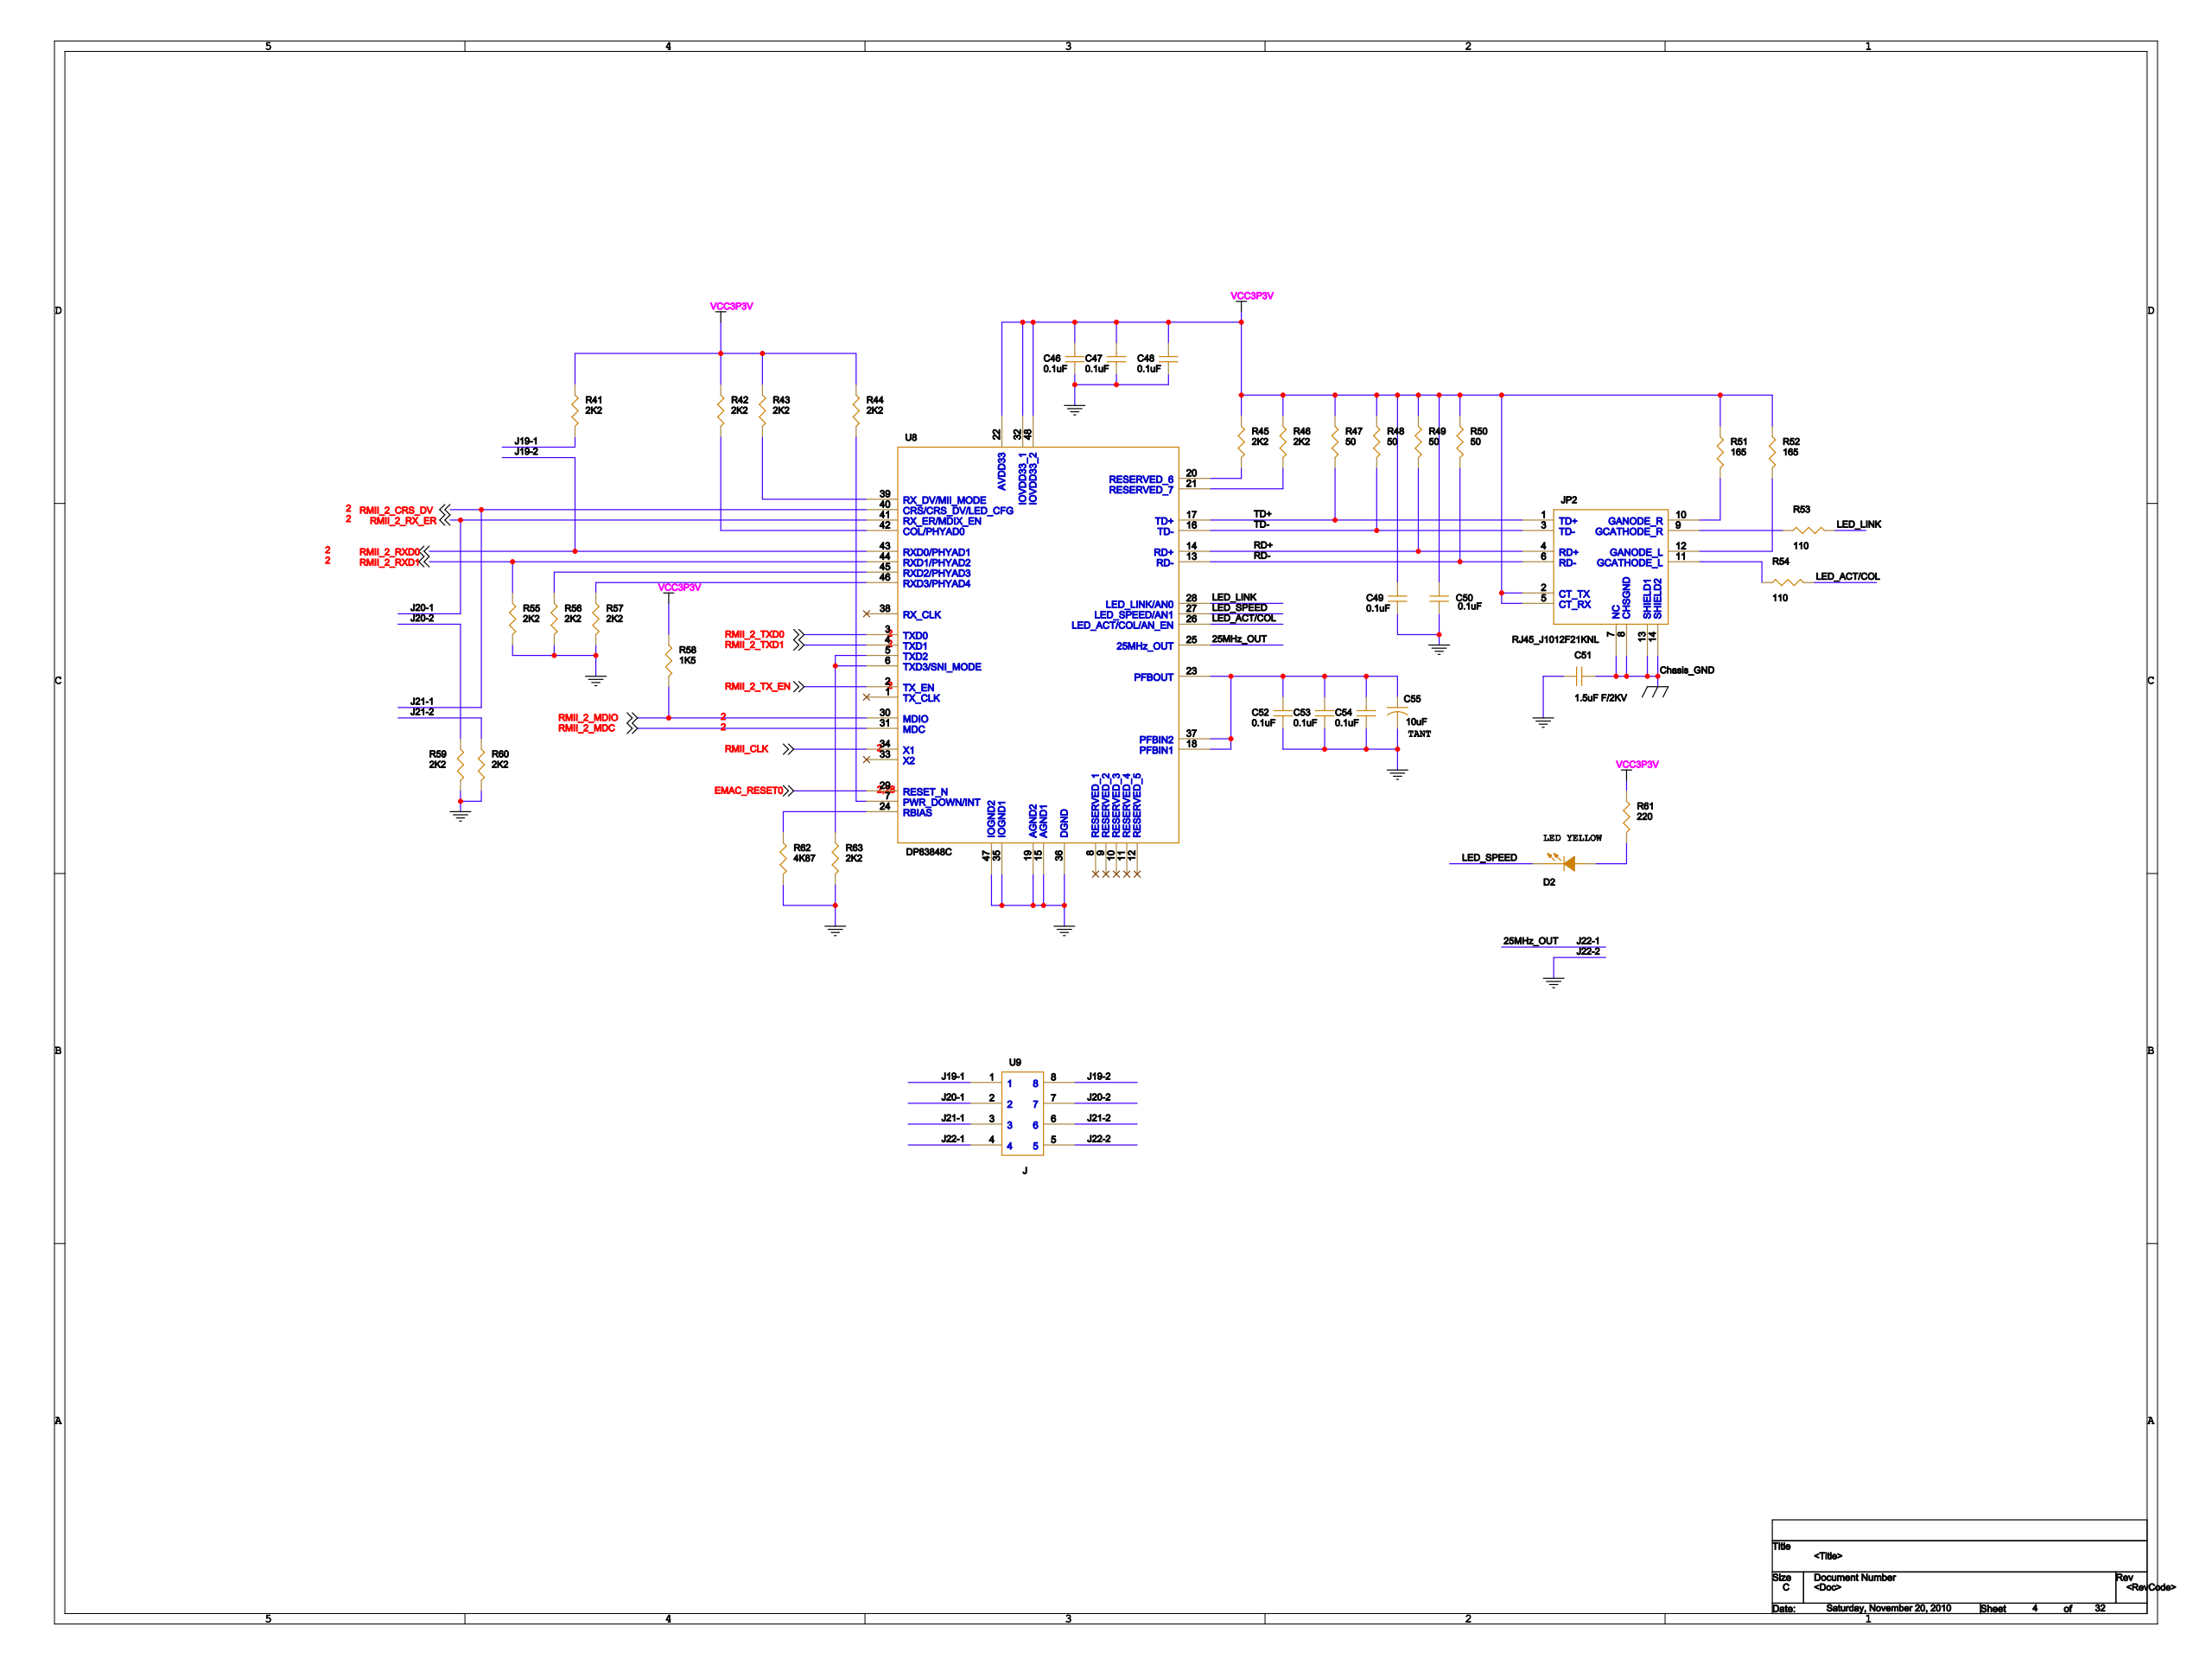Circuit board | Cadence Allegro | 1001 parts | 1318 nets | one sheet of the schematic
Parts on this sheet (reference | value | footprint):
C46 | 0.1uF | 0603
C47 | 0.1uF | 0603
C48 | 0.1uF | 0603
C49 | 0.1uF | 0603
C51 | 1.5uF F/2KV | 0603
C52 | 0.1uF | 0603
C53 | 0.1uF | 0603
C54 | 0.1uF | 0603
C55 | 10uF | C1206
D2 | LED YELLOW | LED0805
JP2 | RJ45_J1012F21KNL | RJ45_J1012F21KNL
R41 | 2K2 | 0603
R42 | 2K2 | 0603
R43 | 2K2 | 0603
R44 | 2K2 | 0603
R45 | 2K2 | 0603
R46 | 2K2 | 0603
R47 | 50 | 0603
R48 | 50 | 0603
R49 | 50 | 0603
R50 | 50 | 0603
R51 | 165 | 0603
R52 | 165 | 0603
R53 | 110 | 0603
R54 | 110 | 0603
R55 | 2K2 | 0603
R56 | 2K2 | 0603
R57 | 2K2 | 0603
R58 | 1K5 | 0603
R59 | 2K2 | 0603
R60 | 2K2 | 0603
R61 | 220 | 0603
R62 | 4K87 | 0603
R63 | 2K2 | 0603
U8 | DP83848C | DP83848C_48LQFP
U9 | J | CON2X4
Nets of these parts (net: part-pin ...):
EMAC_RESET0: U8-29
GND: C46-1 C47-1 C48-1 C49-1 C51-1 C52-1 C53-1 C54-1 C55-2 R55-2 R56-2 R57-2 R59-2 R60-2 R62-2 R63-2 U9-5 U8-15 U8-19 U8-35 U8-36 U8-47
VCC3P3V: C46-2 C47-2 C48-2 C49-2 JP2-2 JP2-5 R41-1 R42-1 R43-1 R44-1 R45-1 R46-1 R47-1 R48-1 R49-1 R50-1 R51-1 R52-1 R58-1 R61-1 U8-22 U8-32 U8-48
RMII_2_MDC: U8-31
RMII_2_MDIO: R58-2 U8-30
RMII_CLK: U8-34
RMII_2_CRS_DV: U9-3 U8-40
RMII_2_RXD0: U9-8 U8-43
RMII_2_RXD1: R55-1 U8-44
RMII_2_RX_ER: U9-2 U8-41
RMII_2_TXD0: U8-3
RMII_2_TXD1: U8-4
RMII_2_TX_EN: U8-2
N16259418: C52-2 C53-2 C54-2 C55-1 U8-18 U8-23 U8-37
CHASIS_GND: C51-2 JP2-7 JP2-8 JP2-13 JP2-14
N16260070: D2-1 R61-2
LED_SPEED: D2-2 U8-27
N16259350: JP2-12 R52-2
N16259982: JP2-10 R51-2
N16259858: JP2-11 R54-1
N16259768: JP2-9 R53-1
RD+: JP2-4 R49-2 U8-14
RD-: JP2-6 R50-2 U8-13
TD+: JP2-1 R47-2 U8-17
TD-: JP2-3 R48-2 U8-16
J19-1: R41-2 U9-1
N16259730: R42-2 U8-42
N16259496: R43-2 U8-39
N16259974: R44-2 U8-7
N16259602: R45-2 U8-20
N16259790: R46-2 U8-21
N16260050: R56-1 U8-45
N16259944: R57-1 U8-46
J20-2: R59-1 U9-7
J21-2: R60-1 U9-6
N16259390: R63-1 U8-5 U8-6
LED_LINK: R53-2 U8-28
LED_ACT/COL: R54-2 U8-26
N16259662: R62-1 U8-24
25MHZ_OUT: U9-4 U8-25